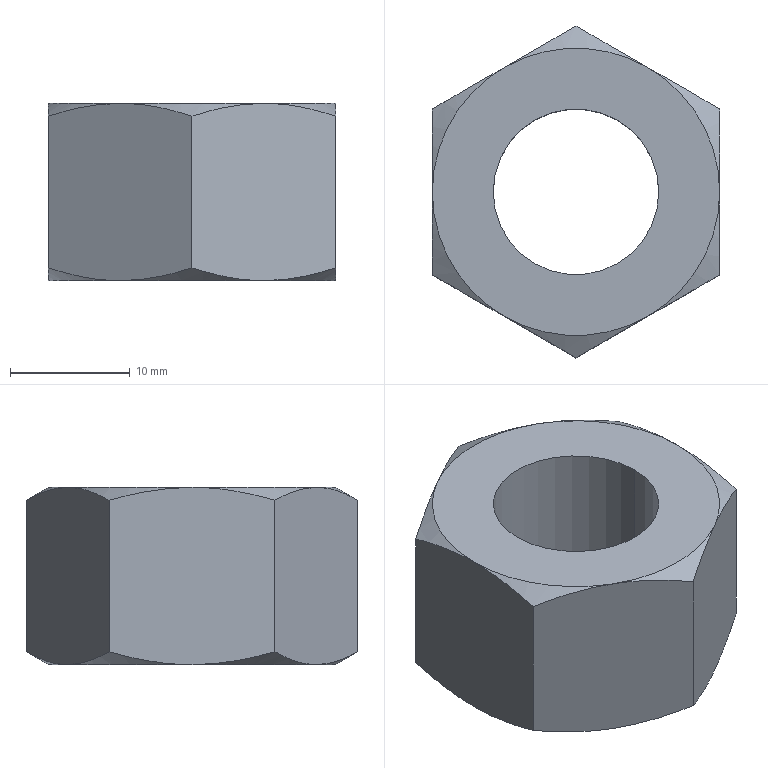Part | SolidWorks | features Cut 2, Extrusion 1 | 1 solid | 22 faces | box 24 x 27.713 x 14.8 mm | volume 5128 mm3 | cone 12 | plane 8 | cylinder 2 | commonest cylinder face diameters 13.835 x2
STEP:
#1=CARTESIAN_POINT('',(-6.918,0.,14.8));
#2=VERTEX_POINT('',#1);
#3=CARTESIAN_POINT('',(6.918,0.,14.8));
#4=VERTEX_POINT('',#3);
#5=CARTESIAN_POINT('',(0.,0.,14.8));
#6=DIRECTION('',(0.,0.,1.));
#7=DIRECTION('',(1.,0.,0.));
#8=AXIS2_PLACEMENT_3D('',#5,#6,#7);
#9=CIRCLE('',#8,6.918);
#10=EDGE_CURVE('',#2,#4,#9,.T.);
#11=ORIENTED_EDGE('',*,*,#10,.T.);
#12=CARTESIAN_POINT('',(6.918,0.,0.));
#13=VERTEX_POINT('',#12);
#14=CARTESIAN_POINT('',(6.918,0.,14.8));
#15=DIRECTION('',(0.,0.,-1.));
#16=VECTOR('',#15,1000.);
#17=LINE('',#14,#16);
#18=EDGE_CURVE('',#4,#13,#17,.T.);
#19=ORIENTED_EDGE('',*,*,#18,.T.);
#20=CARTESIAN_POINT('',(-6.918,0.,0.));
#21=VERTEX_POINT('',#20);
#22=CARTESIAN_POINT('',(0.,0.,0.));
#23=DIRECTION('',(0.,0.,1.));
#24=DIRECTION('',(1.,0.,0.));
#25=AXIS2_PLACEMENT_3D('',#22,#23,#24);
#26=CIRCLE('',#25,6.918);
#27=EDGE_CURVE('',#21,#13,#26,.T.);
#28=ORIENTED_EDGE('',*,*,#27,.F.);
#29=CARTESIAN_POINT('',(-6.918,0.,14.8));
#30=DIRECTION('',(0.,0.,-1.));
#31=VECTOR('',#30,1000.);
#32=LINE('',#29,#31);
#33=EDGE_CURVE('',#2,#21,#32,.T.);
#34=ORIENTED_EDGE('',*,*,#33,.F.);
#35=EDGE_LOOP('',(#11,#19,#28,#34));
#36=FACE_OUTER_BOUND('',#35,.T.);
#37=CARTESIAN_POINT('',(0.,0.,14.8));
#38=DIRECTION('',(0.,0.,-1.));
#39=DIRECTION('',(-1.,0.,0.));
#40=AXIS2_PLACEMENT_3D('',#37,#38,#39);
#41=CYLINDRICAL_SURFACE('',#40,6.918);
#42=ADVANCED_FACE('',(#36),#41,.F.);
#43=CARTESIAN_POINT('',(12.,6.928,13.728));
#44=VERTEX_POINT('',#43);
#45=CARTESIAN_POINT('',(6.,10.392,14.8));
#46=VERTEX_POINT('',#45);
#47=CARTESIAN_POINT('',(12.,6.928,13.728));
#48=CARTESIAN_POINT('',(11.018,7.495,14.055));
#49=CARTESIAN_POINT('',(10.03,8.066,14.325));
#50=CARTESIAN_POINT('',(8.032,9.219,14.698));
#51=CARTESIAN_POINT('',(7.022,9.802,14.8));
#52=CARTESIAN_POINT('',(6.,10.392,14.8));
#53=B_SPLINE_CURVE_WITH_KNOTS('',3,(#47,#48,#49,#50,#51,#52),.UNSPECIFIED.,.F.,.F.,(4,2,4),(0.000000238,0.003505,0.00701),.UNSPECIFIED.);
#54=EDGE_CURVE('',#44,#46,#53,.T.);
#55=ORIENTED_EDGE('',*,*,#54,.F.);
#56=CARTESIAN_POINT('',(12.,6.928,1.072));
#57=VERTEX_POINT('',#56);
#58=CARTESIAN_POINT('',(12.,6.928,14.8));
#59=DIRECTION('',(0.,0.,-1.));
#60=VECTOR('',#59,1000.);
#61=LINE('',#58,#60);
#62=EDGE_CURVE('',#44,#57,#61,.T.);
#63=ORIENTED_EDGE('',*,*,#62,.T.);
#64=CARTESIAN_POINT('',(6.,10.392,0.));
#65=VERTEX_POINT('',#64);
#66=CARTESIAN_POINT('',(6.,10.392,0.));
#67=CARTESIAN_POINT('',(6.509,10.098,0.));
#68=CARTESIAN_POINT('',(7.021,9.803,0.02533));
#69=CARTESIAN_POINT('',(8.033,9.219,0.1234));
#70=CARTESIAN_POINT('',(8.535,8.929,0.196));
#71=CARTESIAN_POINT('',(10.034,8.063,0.476));
#72=CARTESIAN_POINT('',(11.021,7.493,0.7454));
#73=CARTESIAN_POINT('',(12.,6.928,1.072));
#74=B_SPLINE_CURVE_WITH_KNOTS('',3,(#66,#67,#68,#69,#70,#71,#72,#73),.UNSPECIFIED.,.F.,.F.,(4,2,2,4),(0.00701,0.008756,0.0105,0.01399),.UNSPECIFIED.);
#75=EDGE_CURVE('',#65,#57,#74,.T.);
#76=ORIENTED_EDGE('',*,*,#75,.F.);
#77=CARTESIAN_POINT('',(0.,13.856,1.072));
#78=VERTEX_POINT('',#77);
#79=CARTESIAN_POINT('',(0.,13.856,1.072));
#80=CARTESIAN_POINT('',(0.9815,13.29,0.7446));
#81=CARTESIAN_POINT('',(1.97,12.719,0.4751));
#82=CARTESIAN_POINT('',(3.968,11.565,0.1021));
#83=CARTESIAN_POINT('',(4.978,10.982,0.));
#84=CARTESIAN_POINT('',(6.,10.392,0.));
#85=B_SPLINE_CURVE_WITH_KNOTS('',3,(#79,#80,#81,#82,#83,#84),.UNSPECIFIED.,.F.,.F.,(4,2,4),(0.000000238,0.003505,0.00701),.UNSPECIFIED.);
#86=EDGE_CURVE('',#78,#65,#85,.T.);
#87=ORIENTED_EDGE('',*,*,#86,.F.);
#88=CARTESIAN_POINT('',(0.,13.856,13.728));
#89=VERTEX_POINT('',#88);
#90=CARTESIAN_POINT('',(0.,13.856,14.8));
#91=DIRECTION('',(0.,0.,-1.));
#92=VECTOR('',#91,1000.);
#93=LINE('',#90,#92);
#94=EDGE_CURVE('',#89,#78,#93,.T.);
#95=ORIENTED_EDGE('',*,*,#94,.F.);
#96=CARTESIAN_POINT('',(6.,10.392,14.8));
#97=CARTESIAN_POINT('',(5.491,10.686,14.8));
#98=CARTESIAN_POINT('',(4.979,10.982,14.775));
#99=CARTESIAN_POINT('',(3.967,11.566,14.677));
#100=CARTESIAN_POINT('',(3.465,11.856,14.604));
#101=CARTESIAN_POINT('',(1.966,12.721,14.324));
#102=CARTESIAN_POINT('',(0.9791,13.291,14.055));
#103=CARTESIAN_POINT('',(0.,13.856,13.728));
#104=B_SPLINE_CURVE_WITH_KNOTS('',3,(#96,#97,#98,#99,#100,#101,#102,#103),.UNSPECIFIED.,.F.,.F.,(4,2,2,4),(0.00701,0.008756,0.0105,0.01399),.UNSPECIFIED.);
#105=EDGE_CURVE('',#46,#89,#104,.T.);
#106=ORIENTED_EDGE('',*,*,#105,.F.);
#107=EDGE_LOOP('',(#55,#63,#76,#87,#95,#106));
#108=FACE_OUTER_BOUND('',#107,.T.);
#109=CARTESIAN_POINT('',(12.,6.928,14.8));
#110=DIRECTION('',(-0.5,-0.866,0.));
#111=DIRECTION('',(0.866,-0.5,0.));
#112=AXIS2_PLACEMENT_3D('',#109,#110,#111);
#113=PLANE('',#112);
#114=ADVANCED_FACE('',(#108),#113,.F.);
#115=CARTESIAN_POINT('',(-6.,10.392,14.8));
#116=VERTEX_POINT('',#115);
#117=CARTESIAN_POINT('',(0.,13.856,13.728));
#118=CARTESIAN_POINT('',(-0.9815,13.29,14.055));
#119=CARTESIAN_POINT('',(-1.97,12.719,14.325));
#120=CARTESIAN_POINT('',(-3.968,11.565,14.698));
#121=CARTESIAN_POINT('',(-4.978,10.982,14.8));
#122=CARTESIAN_POINT('',(-6.,10.392,14.8));
#123=B_SPLINE_CURVE_WITH_KNOTS('',3,(#117,#118,#119,#120,#121,#122),.UNSPECIFIED.,.F.,.F.,(4,2,4),(0.000000238,0.003505,0.00701),.UNSPECIFIED.);
#124=EDGE_CURVE('',#89,#116,#123,.T.);
#125=ORIENTED_EDGE('',*,*,#124,.F.);
#126=ORIENTED_EDGE('',*,*,#94,.T.);
#127=CARTESIAN_POINT('',(-6.,10.392,0.));
#128=VERTEX_POINT('',#127);
#129=CARTESIAN_POINT('',(-6.,10.392,0.));
#130=CARTESIAN_POINT('',(-5.491,10.686,0.));
#131=CARTESIAN_POINT('',(-4.979,10.982,0.02533));
#132=CARTESIAN_POINT('',(-3.967,11.566,0.1234));
#133=CARTESIAN_POINT('',(-3.465,11.856,0.196));
#134=CARTESIAN_POINT('',(-1.966,12.721,0.476));
#135=CARTESIAN_POINT('',(-0.9791,13.291,0.7454));
#136=CARTESIAN_POINT('',(0.,13.856,1.072));
#137=B_SPLINE_CURVE_WITH_KNOTS('',3,(#129,#130,#131,#132,#133,#134,#135,#136),.UNSPECIFIED.,.F.,.F.,(4,2,2,4),(0.00701,0.008756,0.0105,0.01399),.UNSPECIFIED.);
#138=EDGE_CURVE('',#128,#78,#137,.T.);
#139=ORIENTED_EDGE('',*,*,#138,.F.);
#140=CARTESIAN_POINT('',(-12.,6.928,1.072));
#141=VERTEX_POINT('',#140);
#142=CARTESIAN_POINT('',(-12.,6.928,1.072));
#143=CARTESIAN_POINT('',(-11.018,7.495,0.7446));
#144=CARTESIAN_POINT('',(-10.03,8.066,0.4751));
#145=CARTESIAN_POINT('',(-8.032,9.219,0.1021));
#146=CARTESIAN_POINT('',(-7.022,9.802,0.));
#147=CARTESIAN_POINT('',(-6.,10.392,0.));
#148=B_SPLINE_CURVE_WITH_KNOTS('',3,(#142,#143,#144,#145,#146,#147),.UNSPECIFIED.,.F.,.F.,(4,2,4),(0.000000238,0.003505,0.00701),.UNSPECIFIED.);
#149=EDGE_CURVE('',#141,#128,#148,.T.);
#150=ORIENTED_EDGE('',*,*,#149,.F.);
#151=CARTESIAN_POINT('',(-12.,6.928,13.728));
#152=VERTEX_POINT('',#151);
#153=CARTESIAN_POINT('',(-12.,6.928,14.8));
#154=DIRECTION('',(0.,0.,-1.));
#155=VECTOR('',#154,1000.);
#156=LINE('',#153,#155);
#157=EDGE_CURVE('',#152,#141,#156,.T.);
#158=ORIENTED_EDGE('',*,*,#157,.F.);
#159=CARTESIAN_POINT('',(-6.,10.392,14.8));
#160=CARTESIAN_POINT('',(-6.509,10.098,14.8));
#161=CARTESIAN_POINT('',(-7.021,9.803,14.775));
#162=CARTESIAN_POINT('',(-8.033,9.219,14.677));
#163=CARTESIAN_POINT('',(-8.535,8.929,14.604));
#164=CARTESIAN_POINT('',(-10.034,8.063,14.324));
#165=CARTESIAN_POINT('',(-11.021,7.493,14.055));
#166=CARTESIAN_POINT('',(-12.,6.928,13.728));
#167=B_SPLINE_CURVE_WITH_KNOTS('',3,(#159,#160,#161,#162,#163,#164,#165,#166),.UNSPECIFIED.,.F.,.F.,(4,2,2,4),(0.00701,0.008756,0.0105,0.01399),.UNSPECIFIED.);
#168=EDGE_CURVE('',#116,#152,#167,.T.);
#169=ORIENTED_EDGE('',*,*,#168,.F.);
#170=EDGE_LOOP('',(#125,#126,#139,#150,#158,#169));
#171=FACE_OUTER_BOUND('',#170,.T.);
#172=CARTESIAN_POINT('',(0.,13.856,14.8));
#173=DIRECTION('',(0.5,-0.866,0.));
#174=DIRECTION('',(0.866,0.5,0.));
#175=AXIS2_PLACEMENT_3D('',#172,#173,#174);
#176=PLANE('',#175);
#177=ADVANCED_FACE('',(#171),#176,.F.);
#178=CARTESIAN_POINT('',(-12.,0.,14.8));
#179=VERTEX_POINT('',#178);
#180=CARTESIAN_POINT('',(-12.,6.928,13.728));
#181=CARTESIAN_POINT('',(-12.,5.808,14.052));
#182=CARTESIAN_POINT('',(-12.,4.673,14.321));
#183=CARTESIAN_POINT('',(-12.,2.939,14.602));
#184=CARTESIAN_POINT('',(-12.,2.355,14.676));
#185=CARTESIAN_POINT('',(-12.,1.175,14.775));
#186=CARTESIAN_POINT('',(-12.,0.5863,14.8));
#187=CARTESIAN_POINT('',(-12.,0.,14.8));
#188=B_SPLINE_CURVE_WITH_KNOTS('',3,(#180,#181,#182,#183,#184,#185,#186,#187),.UNSPECIFIED.,.F.,.F.,(4,2,2,4),(0.03963,0.04314,0.04489,0.04664),.UNSPECIFIED.);
#189=EDGE_CURVE('',#152,#179,#188,.T.);
#190=ORIENTED_EDGE('',*,*,#189,.F.);
#191=ORIENTED_EDGE('',*,*,#157,.T.);
#192=CARTESIAN_POINT('',(-12.,0.,0.));
#193=VERTEX_POINT('',#192);
#194=CARTESIAN_POINT('',(-12.,0.,0.));
#195=CARTESIAN_POINT('',(-12.,0.5863,0.));
#196=CARTESIAN_POINT('',(-12.,1.175,0.025));
#197=CARTESIAN_POINT('',(-12.,2.355,0.1241));
#198=CARTESIAN_POINT('',(-12.,2.939,0.1975));
#199=CARTESIAN_POINT('',(-12.,4.673,0.4791));
#200=CARTESIAN_POINT('',(-12.,5.808,0.7483));
#201=CARTESIAN_POINT('',(-12.,6.928,1.072));
#202=B_SPLINE_CURVE_WITH_KNOTS('',3,(#194,#195,#196,#197,#198,#199,#200,#201),.UNSPECIFIED.,.F.,.F.,(4,2,2,4),(0.01971,0.02147,0.02322,0.02673),.UNSPECIFIED.);
#203=EDGE_CURVE('',#193,#141,#202,.T.);
#204=ORIENTED_EDGE('',*,*,#203,.F.);
#205=CARTESIAN_POINT('',(-12.,-6.928,1.072));
#206=VERTEX_POINT('',#205);
#207=CARTESIAN_POINT('',(-12.,-6.928,1.072));
#208=CARTESIAN_POINT('',(-12.,-5.8,0.7462));
#209=CARTESIAN_POINT('',(-12.,-4.647,0.4736));
#210=CARTESIAN_POINT('',(-12.,-2.335,0.1008));
#211=CARTESIAN_POINT('',(-12.,-1.172,0.));
#212=CARTESIAN_POINT('',(-12.,0.,0.));
#213=B_SPLINE_CURVE_WITH_KNOTS('',3,(#207,#208,#209,#210,#211,#212),.UNSPECIFIED.,.F.,.F.,(4,2,4),(0.0127,0.01621,0.01971),.UNSPECIFIED.);
#214=EDGE_CURVE('',#206,#193,#213,.T.);
#215=ORIENTED_EDGE('',*,*,#214,.F.);
#216=CARTESIAN_POINT('',(-12.,-6.928,13.728));
#217=VERTEX_POINT('',#216);
#218=CARTESIAN_POINT('',(-12.,-6.928,14.8));
#219=DIRECTION('',(0.,0.,-1.));
#220=VECTOR('',#219,1000.);
#221=LINE('',#218,#220);
#222=EDGE_CURVE('',#217,#206,#221,.T.);
#223=ORIENTED_EDGE('',*,*,#222,.F.);
#224=CARTESIAN_POINT('',(-12.,0.,14.8));
#225=CARTESIAN_POINT('',(-12.,-1.172,14.8));
#226=CARTESIAN_POINT('',(-12.,-2.335,14.699));
#227=CARTESIAN_POINT('',(-12.,-4.647,14.326));
#228=CARTESIAN_POINT('',(-12.,-5.8,14.054));
#229=CARTESIAN_POINT('',(-12.,-6.928,13.728));
#230=B_SPLINE_CURVE_WITH_KNOTS('',3,(#224,#225,#226,#227,#228,#229),.UNSPECIFIED.,.F.,.F.,(4,2,4),(0.04664,0.05015,0.05365),.UNSPECIFIED.);
#231=EDGE_CURVE('',#179,#217,#230,.T.);
#232=ORIENTED_EDGE('',*,*,#231,.F.);
#233=EDGE_LOOP('',(#190,#191,#204,#215,#223,#232));
#234=FACE_OUTER_BOUND('',#233,.T.);
#235=CARTESIAN_POINT('',(-12.,6.928,14.8));
#236=DIRECTION('',(1.,0.,0.));
#237=DIRECTION('',(0.,1.,0.));
#238=AXIS2_PLACEMENT_3D('',#235,#236,#237);
#239=PLANE('',#238);
#240=ADVANCED_FACE('',(#234),#239,.F.);
#241=CARTESIAN_POINT('',(-6.,-10.392,14.8));
#242=VERTEX_POINT('',#241);
#243=CARTESIAN_POINT('',(-12.,-6.928,13.728));
#244=CARTESIAN_POINT('',(-11.018,-7.495,14.055));
#245=CARTESIAN_POINT('',(-10.03,-8.066,14.325));
#246=CARTESIAN_POINT('',(-8.032,-9.219,14.698));
#247=CARTESIAN_POINT('',(-7.022,-9.802,14.8));
#248=CARTESIAN_POINT('',(-6.,-10.392,14.8));
#249=B_SPLINE_CURVE_WITH_KNOTS('',3,(#243,#244,#245,#246,#247,#248),.UNSPECIFIED.,.F.,.F.,(4,2,4),(0.000000238,0.003505,0.00701),.UNSPECIFIED.);
#250=EDGE_CURVE('',#217,#242,#249,.T.);
#251=ORIENTED_EDGE('',*,*,#250,.F.);
#252=ORIENTED_EDGE('',*,*,#222,.T.);
#253=CARTESIAN_POINT('',(-6.,-10.392,0.));
#254=VERTEX_POINT('',#253);
#255=CARTESIAN_POINT('',(-6.,-10.392,0.));
#256=CARTESIAN_POINT('',(-6.509,-10.098,0.));
#257=CARTESIAN_POINT('',(-7.021,-9.803,0.02533));
#258=CARTESIAN_POINT('',(-8.033,-9.219,0.1234));
#259=CARTESIAN_POINT('',(-8.535,-8.929,0.196));
#260=CARTESIAN_POINT('',(-10.034,-8.063,0.476));
#261=CARTESIAN_POINT('',(-11.021,-7.493,0.7454));
#262=CARTESIAN_POINT('',(-12.,-6.928,1.072));
#263=B_SPLINE_CURVE_WITH_KNOTS('',3,(#255,#256,#257,#258,#259,#260,#261,#262),.UNSPECIFIED.,.F.,.F.,(4,2,2,4),(0.00701,0.008756,0.0105,0.01399),.UNSPECIFIED.);
#264=EDGE_CURVE('',#254,#206,#263,.T.);
#265=ORIENTED_EDGE('',*,*,#264,.F.);
#266=CARTESIAN_POINT('',(0.,-13.856,1.072));
#267=VERTEX_POINT('',#266);
#268=CARTESIAN_POINT('',(0.,-13.856,1.072));
#269=CARTESIAN_POINT('',(-0.9815,-13.29,0.7446));
#270=CARTESIAN_POINT('',(-1.97,-12.719,0.4751));
#271=CARTESIAN_POINT('',(-3.968,-11.565,0.1021));
#272=CARTESIAN_POINT('',(-4.978,-10.982,0.));
#273=CARTESIAN_POINT('',(-6.,-10.392,0.));
#274=B_SPLINE_CURVE_WITH_KNOTS('',3,(#268,#269,#270,#271,#272,#273),.UNSPECIFIED.,.F.,.F.,(4,2,4),(0.000000238,0.003505,0.00701),.UNSPECIFIED.);
#275=EDGE_CURVE('',#267,#254,#274,.T.);
#276=ORIENTED_EDGE('',*,*,#275,.F.);
#277=CARTESIAN_POINT('',(0.,-13.856,13.728));
#278=VERTEX_POINT('',#277);
#279=CARTESIAN_POINT('',(0.,-13.856,14.8));
#280=DIRECTION('',(0.,0.,-1.));
#281=VECTOR('',#280,1000.);
#282=LINE('',#279,#281);
#283=EDGE_CURVE('',#278,#267,#282,.T.);
#284=ORIENTED_EDGE('',*,*,#283,.F.);
#285=CARTESIAN_POINT('',(-6.,-10.392,14.8));
#286=CARTESIAN_POINT('',(-5.491,-10.686,14.8));
#287=CARTESIAN_POINT('',(-4.979,-10.982,14.775));
#288=CARTESIAN_POINT('',(-3.967,-11.566,14.677));
#289=CARTESIAN_POINT('',(-3.465,-11.856,14.604));
#290=CARTESIAN_POINT('',(-1.966,-12.721,14.324));
#291=CARTESIAN_POINT('',(-0.9791,-13.291,14.055));
#292=CARTESIAN_POINT('',(0.,-13.856,13.728));
#293=B_SPLINE_CURVE_WITH_KNOTS('',3,(#285,#286,#287,#288,#289,#290,#291,#292),.UNSPECIFIED.,.F.,.F.,(4,2,2,4),(0.00701,0.008756,0.0105,0.01399),.UNSPECIFIED.);
#294=EDGE_CURVE('',#242,#278,#293,.T.);
#295=ORIENTED_EDGE('',*,*,#294,.F.);
#296=EDGE_LOOP('',(#251,#252,#265,#276,#284,#295));
#297=FACE_OUTER_BOUND('',#296,.T.);
#298=CARTESIAN_POINT('',(-12.,-6.928,14.8));
#299=DIRECTION('',(0.5,0.866,0.));
#300=DIRECTION('',(-0.866,0.5,0.));
#301=AXIS2_PLACEMENT_3D('',#298,#299,#300);
#302=PLANE('',#301);
#303=ADVANCED_FACE('',(#297),#302,.F.);
#304=CARTESIAN_POINT('',(6.,-10.392,14.8));
#305=VERTEX_POINT('',#304);
#306=CARTESIAN_POINT('',(0.,-13.856,13.728));
#307=CARTESIAN_POINT('',(0.9815,-13.29,14.055));
#308=CARTESIAN_POINT('',(1.97,-12.719,14.325));
#309=CARTESIAN_POINT('',(3.968,-11.565,14.698));
#310=CARTESIAN_POINT('',(4.978,-10.982,14.8));
#311=CARTESIAN_POINT('',(6.,-10.392,14.8));
#312=B_SPLINE_CURVE_WITH_KNOTS('',3,(#306,#307,#308,#309,#310,#311),.UNSPECIFIED.,.F.,.F.,(4,2,4),(0.000000238,0.003505,0.00701),.UNSPECIFIED.);
#313=EDGE_CURVE('',#278,#305,#312,.T.);
#314=ORIENTED_EDGE('',*,*,#313,.F.);
#315=ORIENTED_EDGE('',*,*,#283,.T.);
#316=CARTESIAN_POINT('',(6.,-10.392,0.));
#317=VERTEX_POINT('',#316);
#318=CARTESIAN_POINT('',(6.,-10.392,0.));
#319=CARTESIAN_POINT('',(5.491,-10.686,0.));
#320=CARTESIAN_POINT('',(4.979,-10.982,0.02533));
#321=CARTESIAN_POINT('',(3.967,-11.566,0.1234));
#322=CARTESIAN_POINT('',(3.465,-11.856,0.196));
#323=CARTESIAN_POINT('',(1.966,-12.721,0.476));
#324=CARTESIAN_POINT('',(0.9791,-13.291,0.7454));
#325=CARTESIAN_POINT('',(0.,-13.856,1.072));
#326=B_SPLINE_CURVE_WITH_KNOTS('',3,(#318,#319,#320,#321,#322,#323,#324,#325),.UNSPECIFIED.,.F.,.F.,(4,2,2,4),(0.00701,0.008756,0.0105,0.01399),.UNSPECIFIED.);
#327=EDGE_CURVE('',#317,#267,#326,.T.);
#328=ORIENTED_EDGE('',*,*,#327,.F.);
#329=CARTESIAN_POINT('',(12.,-6.928,1.072));
#330=VERTEX_POINT('',#329);
#331=CARTESIAN_POINT('',(12.,-6.928,1.072));
#332=CARTESIAN_POINT('',(11.018,-7.495,0.7446));
#333=CARTESIAN_POINT('',(10.03,-8.066,0.4751));
#334=CARTESIAN_POINT('',(8.032,-9.219,0.1021));
#335=CARTESIAN_POINT('',(7.022,-9.802,0.));
#336=CARTESIAN_POINT('',(6.,-10.392,0.));
#337=B_SPLINE_CURVE_WITH_KNOTS('',3,(#331,#332,#333,#334,#335,#336),.UNSPECIFIED.,.F.,.F.,(4,2,4),(0.000000238,0.003505,0.00701),.UNSPECIFIED.);
#338=EDGE_CURVE('',#330,#317,#337,.T.);
#339=ORIENTED_EDGE('',*,*,#338,.F.);
#340=CARTESIAN_POINT('',(12.,-6.928,13.728));
#341=VERTEX_POINT('',#340);
#342=CARTESIAN_POINT('',(12.,-6.928,14.8));
#343=DIRECTION('',(0.,0.,-1.));
#344=VECTOR('',#343,1000.);
#345=LINE('',#342,#344);
#346=EDGE_CURVE('',#341,#330,#345,.T.);
#347=ORIENTED_EDGE('',*,*,#346,.F.);
#348=CARTESIAN_POINT('',(6.,-10.392,14.8));
#349=CARTESIAN_POINT('',(6.509,-10.098,14.8));
#350=CARTESIAN_POINT('',(7.021,-9.803,14.775));
#351=CARTESIAN_POINT('',(8.033,-9.219,14.677));
#352=CARTESIAN_POINT('',(8.535,-8.929,14.604));
#353=CARTESIAN_POINT('',(10.034,-8.063,14.324));
#354=CARTESIAN_POINT('',(11.021,-7.493,14.055));
#355=CARTESIAN_POINT('',(12.,-6.928,13.728));
#356=B_SPLINE_CURVE_WITH_KNOTS('',3,(#348,#349,#350,#351,#352,#353,#354,#355),.UNSPECIFIED.,.F.,.F.,(4,2,2,4),(0.00701,0.008756,0.0105,0.01399),.UNSPECIFIED.);
#357=EDGE_CURVE('',#305,#341,#356,.T.);
#358=ORIENTED_EDGE('',*,*,#357,.F.);
#359=EDGE_LOOP('',(#314,#315,#328,#339,#347,#358));
#360=FACE_OUTER_BOUND('',#359,.T.);
#361=CARTESIAN_POINT('',(0.,-13.856,14.8));
#362=DIRECTION('',(-0.5,0.866,0.));
#363=DIRECTION('',(-0.866,-0.5,0.));
#364=AXIS2_PLACEMENT_3D('',#361,#362,#363);
#365=PLANE('',#364);
#366=ADVANCED_FACE('',(#360),#365,.F.);
#367=CARTESIAN_POINT('',(12.,0.,14.8));
#368=VERTEX_POINT('',#367);
#369=CARTESIAN_POINT('',(12.,-6.928,13.728));
#370=CARTESIAN_POINT('',(12.,-5.8,14.054));
#371=CARTESIAN_POINT('',(12.,-4.647,14.326));
#372=CARTESIAN_POINT('',(12.,-2.335,14.699));
#373=CARTESIAN_POINT('',(12.,-1.172,14.8));
#374=CARTESIAN_POINT('',(12.,0.,14.8));
#375=B_SPLINE_CURVE_WITH_KNOTS('',3,(#369,#370,#371,#372,#373,#374),.UNSPECIFIED.,.F.,.F.,(4,2,4),(0.0127,0.01621,0.01971),.UNSPECIFIED.);
#376=EDGE_CURVE('',#341,#368,#375,.T.);
#377=ORIENTED_EDGE('',*,*,#376,.F.);
#378=ORIENTED_EDGE('',*,*,#346,.T.);
#379=CARTESIAN_POINT('',(12.,0.,0.));
#380=VERTEX_POINT('',#379);
#381=CARTESIAN_POINT('',(12.,0.,0.));
#382=CARTESIAN_POINT('',(12.,-1.172,0.));
#383=CARTESIAN_POINT('',(12.,-2.335,0.1008));
#384=CARTESIAN_POINT('',(12.,-4.647,0.4736));
#385=CARTESIAN_POINT('',(12.,-5.8,0.7462));
#386=CARTESIAN_POINT('',(12.,-6.928,1.072));
#387=B_SPLINE_CURVE_WITH_KNOTS('',3,(#381,#382,#383,#384,#385,#386),.UNSPECIFIED.,.F.,.F.,(4,2,4),(0.04664,0.05015,0.05365),.UNSPECIFIED.);
#388=EDGE_CURVE('',#380,#330,#387,.T.);
#389=ORIENTED_EDGE('',*,*,#388,.F.);
#390=CARTESIAN_POINT('',(12.,6.928,1.072));
#391=CARTESIAN_POINT('',(12.,5.808,0.7483));
#392=CARTESIAN_POINT('',(12.,4.673,0.4791));
#393=CARTESIAN_POINT('',(12.,2.939,0.1975));
#394=CARTESIAN_POINT('',(12.,2.355,0.1241));
#395=CARTESIAN_POINT('',(12.,1.175,0.025));
#396=CARTESIAN_POINT('',(12.,0.5863,0.));
#397=CARTESIAN_POINT('',(12.,0.,0.));
#398=B_SPLINE_CURVE_WITH_KNOTS('',3,(#390,#391,#392,#393,#394,#395,#396,#397),.UNSPECIFIED.,.F.,.F.,(4,2,2,4),(0.03963,0.04314,0.04489,0.04664),.UNSPECIFIED.);
#399=EDGE_CURVE('',#57,#380,#398,.T.);
#400=ORIENTED_EDGE('',*,*,#399,.F.);
#401=ORIENTED_EDGE('',*,*,#62,.F.);
#402=CARTESIAN_POINT('',(12.,0.,14.8));
#403=CARTESIAN_POINT('',(12.,0.5863,14.8));
#404=CARTESIAN_POINT('',(12.,1.175,14.775));
#405=CARTESIAN_POINT('',(12.,2.355,14.676));
#406=CARTESIAN_POINT('',(12.,2.939,14.602));
#407=CARTESIAN_POINT('',(12.,4.673,14.321));
#408=CARTESIAN_POINT('',(12.,5.808,14.052));
#409=CARTESIAN_POINT('',(12.,6.928,13.728));
#410=B_SPLINE_CURVE_WITH_KNOTS('',3,(#402,#403,#404,#405,#406,#407,#408,#409),.UNSPECIFIED.,.F.,.F.,(4,2,2,4),(0.01971,0.02147,0.02322,0.02673),.UNSPECIFIED.);
#411=EDGE_CURVE('',#368,#44,#410,.T.);
#412=ORIENTED_EDGE('',*,*,#411,.F.);
#413=EDGE_LOOP('',(#377,#378,#389,#400,#401,#412));
#414=FACE_OUTER_BOUND('',#413,.T.);
#415=CARTESIAN_POINT('',(12.,-6.928,14.8));
#416=DIRECTION('',(-1.,0.,0.));
#417=DIRECTION('',(0.,-1.,0.));
#418=AXIS2_PLACEMENT_3D('',#415,#416,#417);
#419=PLANE('',#418);
#420=ADVANCED_FACE('',(#414),#419,.F.);
#421=ORIENTED_EDGE('',*,*,#10,.F.);
#422=CARTESIAN_POINT('',(0.,0.,14.8));
#423=DIRECTION('',(0.,0.,1.));
#424=DIRECTION('',(1.,0.,0.));
#425=AXIS2_PLACEMENT_3D('',#422,#423,#424);
#426=CIRCLE('',#425,6.918);
#427=EDGE_CURVE('',#4,#2,#426,.T.);
#428=ORIENTED_EDGE('',*,*,#427,.F.);
#429=EDGE_LOOP('',(#421,#428));
#430=FACE_BOUND('',#429,.T.);
#431=CARTESIAN_POINT('',(0.,0.,14.8));
#432=DIRECTION('',(0.,0.,1.));
#433=DIRECTION('',(1.,0.,0.));
#434=AXIS2_PLACEMENT_3D('',#431,#432,#433);
#435=CIRCLE('',#434,12.);
#436=EDGE_CURVE('',#305,#368,#435,.T.);
#437=ORIENTED_EDGE('',*,*,#436,.T.);
#438=CARTESIAN_POINT('',(0.,0.,14.8));
#439=DIRECTION('',(0.,0.,1.));
#440=DIRECTION('',(1.,0.,0.));
#441=AXIS2_PLACEMENT_3D('',#438,#439,#440);
#442=CIRCLE('',#441,12.);
#443=EDGE_CURVE('',#368,#46,#442,.T.);
#444=ORIENTED_EDGE('',*,*,#443,.T.);
#445=CARTESIAN_POINT('',(0.,0.,14.8));
#446=DIRECTION('',(0.,0.,1.));
#447=DIRECTION('',(1.,0.,0.));
#448=AXIS2_PLACEMENT_3D('',#445,#446,#447);
#449=CIRCLE('',#448,12.);
#450=EDGE_CURVE('',#46,#116,#449,.T.);
#451=ORIENTED_EDGE('',*,*,#450,.T.);
#452=CARTESIAN_POINT('',(0.,0.,14.8));
#453=DIRECTION('',(0.,0.,1.));
#454=DIRECTION('',(1.,0.,0.));
#455=AXIS2_PLACEMENT_3D('',#452,#453,#454);
#456=CIRCLE('',#455,12.);
#457=EDGE_CURVE('',#116,#179,#456,.T.);
#458=ORIENTED_EDGE('',*,*,#457,.T.);
#459=CARTESIAN_POINT('',(0.,0.,14.8));
#460=DIRECTION('',(0.,0.,1.));
#461=DIRECTION('',(1.,0.,0.));
#462=AXIS2_PLACEMENT_3D('',#459,#460,#461);
#463=CIRCLE('',#462,12.);
#464=EDGE_CURVE('',#179,#242,#463,.T.);
#465=ORIENTED_EDGE('',*,*,#464,.T.);
#466=CARTESIAN_POINT('',(0.,0.,14.8));
#467=DIRECTION('',(0.,0.,1.));
#468=DIRECTION('',(1.,0.,0.));
#469=AXIS2_PLACEMENT_3D('',#466,#467,#468);
#470=CIRCLE('',#469,12.);
#471=EDGE_CURVE('',#242,#305,#470,.T.);
#472=ORIENTED_EDGE('',*,*,#471,.T.);
#473=EDGE_LOOP('',(#437,#444,#451,#458,#465,#472));
#474=FACE_OUTER_BOUND('',#473,.T.);
#475=CARTESIAN_POINT('',(-12.,20.785,14.8));
#476=DIRECTION('',(0.,0.,1.));
#477=DIRECTION('',(1.,0.,0.));
#478=AXIS2_PLACEMENT_3D('',#475,#476,#477);
#479=PLANE('',#478);
#480=ADVANCED_FACE('',(#430,#474),#479,.T.);
#481=ORIENTED_EDGE('',*,*,#27,.T.);
#482=CARTESIAN_POINT('',(0.,0.,0.));
#483=DIRECTION('',(0.,0.,1.));
#484=DIRECTION('',(1.,0.,0.));
#485=AXIS2_PLACEMENT_3D('',#482,#483,#484);
#486=CIRCLE('',#485,6.918);
#487=EDGE_CURVE('',#13,#21,#486,.T.);
#488=ORIENTED_EDGE('',*,*,#487,.T.);
#489=EDGE_LOOP('',(#481,#488));
#490=FACE_BOUND('',#489,.T.);
#491=CARTESIAN_POINT('',(0.,0.,0.));
#492=DIRECTION('',(0.,0.,-1.));
#493=DIRECTION('',(-1.,0.,0.));
#494=AXIS2_PLACEMENT_3D('',#491,#492,#493);
#495=CIRCLE('',#494,12.);
#496=EDGE_CURVE('',#65,#380,#495,.T.);
#497=ORIENTED_EDGE('',*,*,#496,.T.);
#498=CARTESIAN_POINT('',(0.,0.,0.));
#499=DIRECTION('',(0.,0.,-1.));
#500=DIRECTION('',(-1.,0.,0.));
#501=AXIS2_PLACEMENT_3D('',#498,#499,#500);
#502=CIRCLE('',#501,12.);
#503=EDGE_CURVE('',#380,#317,#502,.T.);
#504=ORIENTED_EDGE('',*,*,#503,.T.);
#505=CARTESIAN_POINT('',(0.,0.,0.));
#506=DIRECTION('',(0.,0.,-1.));
#507=DIRECTION('',(-1.,0.,0.));
#508=AXIS2_PLACEMENT_3D('',#505,#506,#507);
#509=CIRCLE('',#508,12.);
#510=EDGE_CURVE('',#317,#254,#509,.T.);
#511=ORIENTED_EDGE('',*,*,#510,.T.);
#512=CARTESIAN_POINT('',(0.,0.,0.));
#513=DIRECTION('',(0.,0.,-1.));
#514=DIRECTION('',(-1.,0.,0.));
#515=AXIS2_PLACEMENT_3D('',#512,#513,#514);
#516=CIRCLE('',#515,12.);
#517=EDGE_CURVE('',#254,#193,#516,.T.);
#518=ORIENTED_EDGE('',*,*,#517,.T.);
#519=CARTESIAN_POINT('',(0.,0.,0.));
#520=DIRECTION('',(0.,0.,-1.));
#521=DIRECTION('',(-1.,0.,0.));
#522=AXIS2_PLACEMENT_3D('',#519,#520,#521);
#523=CIRCLE('',#522,12.);
#524=EDGE_CURVE('',#193,#128,#523,.T.);
#525=ORIENTED_EDGE('',*,*,#524,.T.);
#526=CARTESIAN_POINT('',(0.,0.,0.));
#527=DIRECTION('',(0.,0.,-1.));
#528=DIRECTION('',(-1.,0.,0.));
#529=AXIS2_PLACEMENT_3D('',#526,#527,#528);
#530=CIRCLE('',#529,12.);
#531=EDGE_CURVE('',#128,#65,#530,.T.);
#532=ORIENTED_EDGE('',*,*,#531,.T.);
#533=EDGE_LOOP('',(#497,#504,#511,#518,#525,#532));
#534=FACE_OUTER_BOUND('',#533,.T.);
#535=CARTESIAN_POINT('',(-12.,20.785,0.));
#536=DIRECTION('',(0.,0.,1.));
#537=DIRECTION('',(1.,0.,0.));
#538=AXIS2_PLACEMENT_3D('',#535,#536,#537);
#539=PLANE('',#538);
#540=ADVANCED_FACE('',(#490,#534),#539,.F.);
#541=ORIENTED_EDGE('',*,*,#18,.F.);
#542=ORIENTED_EDGE('',*,*,#427,.T.);
#543=ORIENTED_EDGE('',*,*,#33,.T.);
#544=ORIENTED_EDGE('',*,*,#487,.F.);
#545=EDGE_LOOP('',(#541,#542,#543,#544));
#546=FACE_OUTER_BOUND('',#545,.T.);
#547=CARTESIAN_POINT('',(0.,0.,14.8));
#548=DIRECTION('',(0.,0.,-1.));
#549=DIRECTION('',(-1.,0.,0.));
#550=AXIS2_PLACEMENT_3D('',#547,#548,#549);
#551=CYLINDRICAL_SURFACE('',#550,6.918);
#552=ADVANCED_FACE('',(#546),#551,.F.);
#553=ORIENTED_EDGE('',*,*,#338,.T.);
#554=ORIENTED_EDGE('',*,*,#503,.F.);
#555=ORIENTED_EDGE('',*,*,#388,.T.);
#556=EDGE_LOOP('',(#553,#554,#555));
#557=FACE_OUTER_BOUND('',#556,.T.);
#558=CARTESIAN_POINT('',(0.,0.,0.));
#559=DIRECTION('',(0.,0.,1.));
#560=DIRECTION('',(-1.,0.,0.));
#561=AXIS2_PLACEMENT_3D('',#558,#559,#560);
#562=CONICAL_SURFACE('',#561,12.,1.047);
#563=ADVANCED_FACE('',(#557),#562,.T.);
#564=ORIENTED_EDGE('',*,*,#75,.T.);
#565=ORIENTED_EDGE('',*,*,#399,.T.);
#566=ORIENTED_EDGE('',*,*,#496,.F.);
#567=EDGE_LOOP('',(#564,#565,#566));
#568=FACE_OUTER_BOUND('',#567,.T.);
#569=CARTESIAN_POINT('',(0.,0.,0.));
#570=DIRECTION('',(0.,0.,1.));
#571=DIRECTION('',(-1.,0.,0.));
#572=AXIS2_PLACEMENT_3D('',#569,#570,#571);
#573=CONICAL_SURFACE('',#572,12.,1.047);
#574=ADVANCED_FACE('',(#568),#573,.T.);
#575=ORIENTED_EDGE('',*,*,#275,.T.);
#576=ORIENTED_EDGE('',*,*,#510,.F.);
#577=ORIENTED_EDGE('',*,*,#327,.T.);
#578=EDGE_LOOP('',(#575,#576,#577));
#579=FACE_OUTER_BOUND('',#578,.T.);
#580=CARTESIAN_POINT('',(0.,0.,0.));
#581=DIRECTION('',(0.,0.,1.));
#582=DIRECTION('',(-1.,0.,0.));
#583=AXIS2_PLACEMENT_3D('',#580,#581,#582);
#584=CONICAL_SURFACE('',#583,12.,1.047);
#585=ADVANCED_FACE('',(#579),#584,.T.);
#586=ORIENTED_EDGE('',*,*,#214,.T.);
#587=ORIENTED_EDGE('',*,*,#517,.F.);
#588=ORIENTED_EDGE('',*,*,#264,.T.);
#589=EDGE_LOOP('',(#586,#587,#588));
#590=FACE_OUTER_BOUND('',#589,.T.);
#591=CARTESIAN_POINT('',(0.,0.,0.));
#592=DIRECTION('',(0.,0.,1.));
#593=DIRECTION('',(-1.,0.,0.));
#594=AXIS2_PLACEMENT_3D('',#591,#592,#593);
#595=CONICAL_SURFACE('',#594,12.,1.047);
#596=ADVANCED_FACE('',(#590),#595,.T.);
#597=ORIENTED_EDGE('',*,*,#203,.T.);
#598=ORIENTED_EDGE('',*,*,#149,.T.);
#599=ORIENTED_EDGE('',*,*,#524,.F.);
#600=EDGE_LOOP('',(#597,#598,#599));
#601=FACE_OUTER_BOUND('',#600,.T.);
#602=CARTESIAN_POINT('',(0.,0.,0.));
#603=DIRECTION('',(0.,0.,1.));
#604=DIRECTION('',(-1.,0.,0.));
#605=AXIS2_PLACEMENT_3D('',#602,#603,#604);
#606=CONICAL_SURFACE('',#605,12.,1.047);
#607=ADVANCED_FACE('',(#601),#606,.T.);
#608=ORIENTED_EDGE('',*,*,#138,.T.);
#609=ORIENTED_EDGE('',*,*,#86,.T.);
#610=ORIENTED_EDGE('',*,*,#531,.F.);
#611=EDGE_LOOP('',(#608,#609,#610));
#612=FACE_OUTER_BOUND('',#611,.T.);
#613=CARTESIAN_POINT('',(0.,0.,0.));
#614=DIRECTION('',(0.,0.,1.));
#615=DIRECTION('',(-1.,0.,0.));
#616=AXIS2_PLACEMENT_3D('',#613,#614,#615);
#617=CONICAL_SURFACE('',#616,12.,1.047);
#618=ADVANCED_FACE('',(#612),#617,.T.);
#619=ORIENTED_EDGE('',*,*,#357,.T.);
#620=ORIENTED_EDGE('',*,*,#376,.T.);
#621=ORIENTED_EDGE('',*,*,#436,.F.);
#622=EDGE_LOOP('',(#619,#620,#621));
#623=FACE_OUTER_BOUND('',#622,.T.);
#624=CARTESIAN_POINT('',(0.,0.,14.8));
#625=DIRECTION('',(0.,0.,-1.));
#626=DIRECTION('',(1.,0.,0.));
#627=AXIS2_PLACEMENT_3D('',#624,#625,#626);
#628=CONICAL_SURFACE('',#627,12.,1.047);
#629=ADVANCED_FACE('',(#623),#628,.T.);
#630=ORIENTED_EDGE('',*,*,#294,.T.);
#631=ORIENTED_EDGE('',*,*,#313,.T.);
#632=ORIENTED_EDGE('',*,*,#471,.F.);
#633=EDGE_LOOP('',(#630,#631,#632));
#634=FACE_OUTER_BOUND('',#633,.T.);
#635=CARTESIAN_POINT('',(0.,0.,14.8));
#636=DIRECTION('',(0.,0.,-1.));
#637=DIRECTION('',(1.,0.,0.));
#638=AXIS2_PLACEMENT_3D('',#635,#636,#637);
#639=CONICAL_SURFACE('',#638,12.,1.047);
#640=ADVANCED_FACE('',(#634),#639,.T.);
#641=ORIENTED_EDGE('',*,*,#231,.T.);
#642=ORIENTED_EDGE('',*,*,#250,.T.);
#643=ORIENTED_EDGE('',*,*,#464,.F.);
#644=EDGE_LOOP('',(#641,#642,#643));
#645=FACE_OUTER_BOUND('',#644,.T.);
#646=CARTESIAN_POINT('',(0.,0.,14.8));
#647=DIRECTION('',(0.,0.,-1.));
#648=DIRECTION('',(1.,0.,0.));
#649=AXIS2_PLACEMENT_3D('',#646,#647,#648);
#650=CONICAL_SURFACE('',#649,12.,1.047);
#651=ADVANCED_FACE('',(#645),#650,.T.);
#652=ORIENTED_EDGE('',*,*,#168,.T.);
#653=ORIENTED_EDGE('',*,*,#189,.T.);
#654=ORIENTED_EDGE('',*,*,#457,.F.);
#655=EDGE_LOOP('',(#652,#653,#654));
#656=FACE_OUTER_BOUND('',#655,.T.);
#657=CARTESIAN_POINT('',(0.,0.,14.8));
#658=DIRECTION('',(0.,0.,-1.));
#659=DIRECTION('',(1.,0.,0.));
#660=AXIS2_PLACEMENT_3D('',#657,#658,#659);
#661=CONICAL_SURFACE('',#660,12.,1.047);
#662=ADVANCED_FACE('',(#656),#661,.T.);
#663=ORIENTED_EDGE('',*,*,#105,.T.);
#664=ORIENTED_EDGE('',*,*,#124,.T.);
#665=ORIENTED_EDGE('',*,*,#450,.F.);
#666=EDGE_LOOP('',(#663,#664,#665));
#667=FACE_OUTER_BOUND('',#666,.T.);
#668=CARTESIAN_POINT('',(0.,0.,14.8));
#669=DIRECTION('',(0.,0.,-1.));
#670=DIRECTION('',(1.,0.,0.));
#671=AXIS2_PLACEMENT_3D('',#668,#669,#670);
#672=CONICAL_SURFACE('',#671,12.,1.047);
#673=ADVANCED_FACE('',(#667),#672,.T.);
#674=ORIENTED_EDGE('',*,*,#54,.T.);
#675=ORIENTED_EDGE('',*,*,#443,.F.);
#676=ORIENTED_EDGE('',*,*,#411,.T.);
#677=EDGE_LOOP('',(#674,#675,#676));
#678=FACE_OUTER_BOUND('',#677,.T.);
#679=CARTESIAN_POINT('',(0.,0.,14.8));
#680=DIRECTION('',(0.,0.,-1.));
#681=DIRECTION('',(1.,0.,0.));
#682=AXIS2_PLACEMENT_3D('',#679,#680,#681);
#683=CONICAL_SURFACE('',#682,12.,1.047);
#684=ADVANCED_FACE('',(#678),#683,.T.);
#685=CLOSED_SHELL('',(#42,#114,#177,#240,#303,#366,#420,#480,#540,#552,#563,#574,#585,#596,#607,#618,#629,#640,#651,#662,#673,#684));
#686=MANIFOLD_SOLID_BREP('',#685);
#687=CARTESIAN_POINT('',(0.,0.,0.));
#688=DIRECTION('',(0.,0.,1.));
#689=DIRECTION('',(1.,0.,0.));
#690=AXIS2_PLACEMENT_3D('',#687,#688,#689);
#691=(LENGTH_UNIT()NAMED_UNIT(*)SI_UNIT(.MILLI.,.METRE.));
#692=UNCERTAINTY_MEASURE_WITH_UNIT(LENGTH_MEASURE(0.00001),#691,'','');
#693=(NAMED_UNIT(*)PLANE_ANGLE_UNIT()SI_UNIT($,.RADIAN.));
#694=(NAMED_UNIT(*)SI_UNIT($,.STERADIAN.)SOLID_ANGLE_UNIT());
#695=(GEOMETRIC_REPRESENTATION_CONTEXT(3)GLOBAL_UNCERTAINTY_ASSIGNED_CONTEXT((#692))GLOBAL_UNIT_ASSIGNED_CONTEXT((#691,#693,#694))REPRESENTATION_CONTEXT('',''));
#696=ADVANCED_BREP_SHAPE_REPRESENTATION('',(#686,#690),#695);